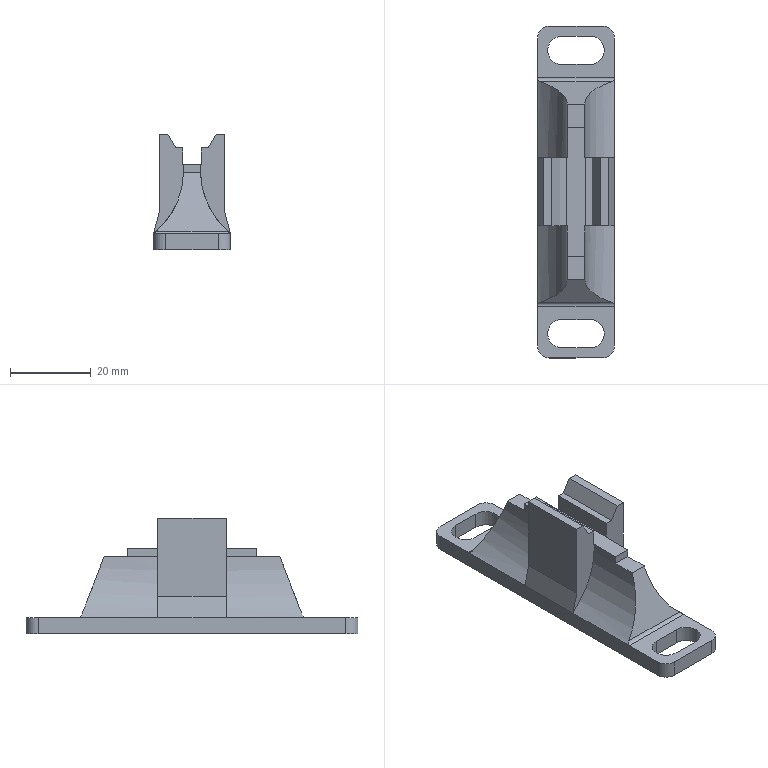Part | STEP file | _Y300T-A_REAR | 1 solid | 54 faces | box 19 x 82 x 28.6 mm | volume 16093 mm3 | plane 38 | cylinder 16 | commonest cylinder face diameters 7 x6 6 x4 40 x4 2 x2